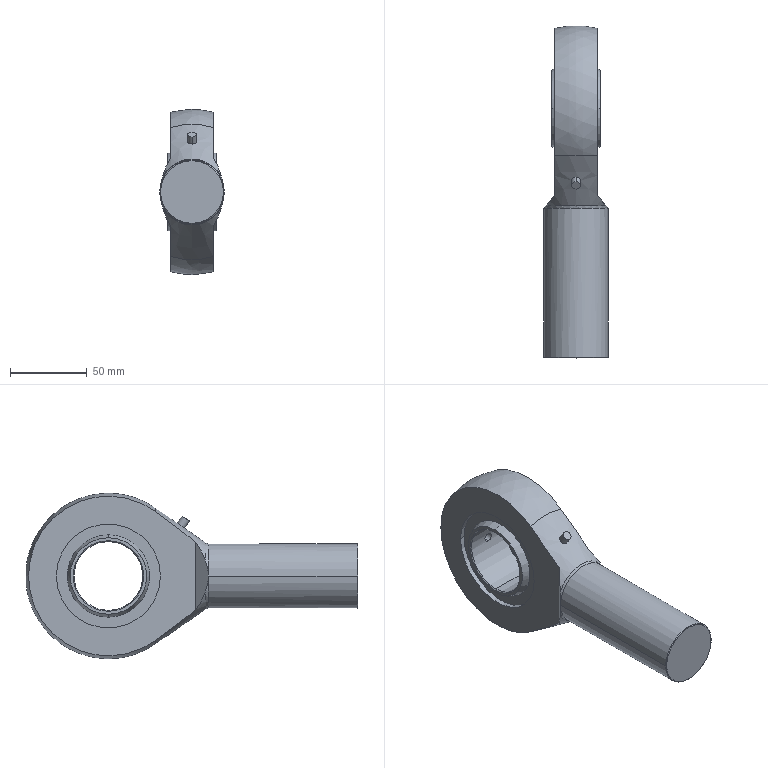Part | SolidWorks | features BaseBody 1 | 1 solid | 41 faces | box 42 x 217 x 108 mm | volume 356904 mm3 | cylinder 14 | plane 12 | cone 8 | spline 7 | commonest cylinder face diameters 5.818 x4 68 x4 5.682 x2 42 x2 45 x2